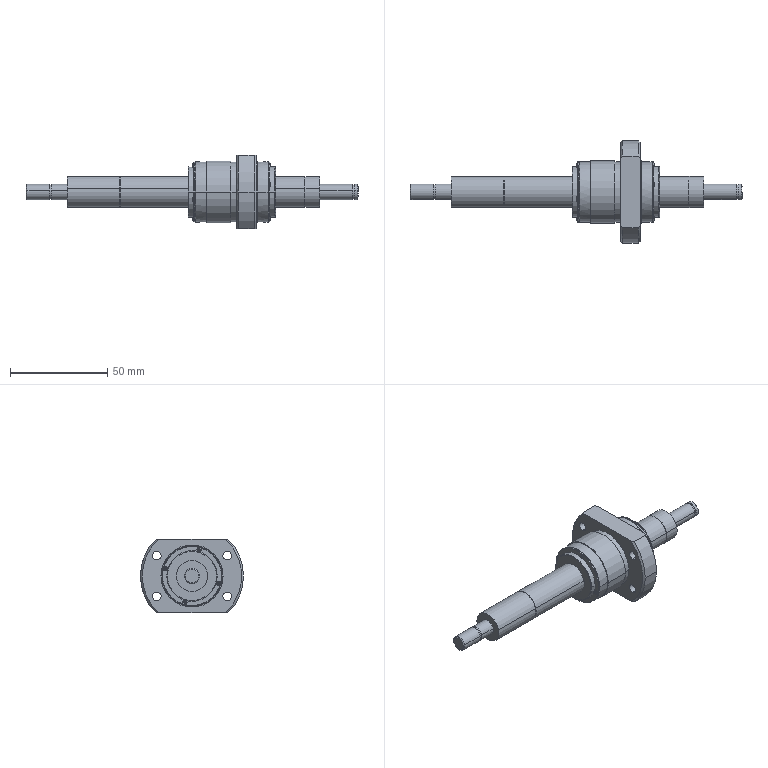Part | SolidWorks | features AEMSimFeature 1 | 2 solids | 228 faces | box 171 x 53 x 38 mm | volume 62164 mm3 | plane 137 | cylinder 71 | cone 16 | torus 4 | commonest cylinder face diameters 2.24 x16 31 x10 4.5 x8 8 x8 16 x8 7.6 x4